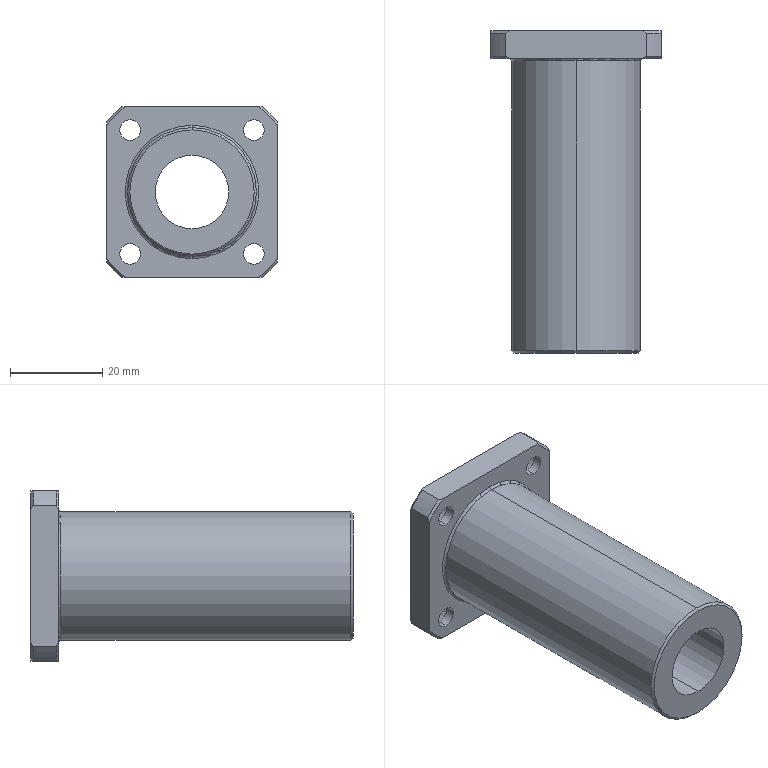Part | STEP file | Bearing LMK16LUU | 1 solid | 49 faces | box 37 x 70 x 37 mm | volume 32483 mm3 | cylinder 24 | cone 12 | plane 11 | torus 2 | commonest cylinder face diameters 4.5 x8 8 x8 48 x4 16 x2 28 x2